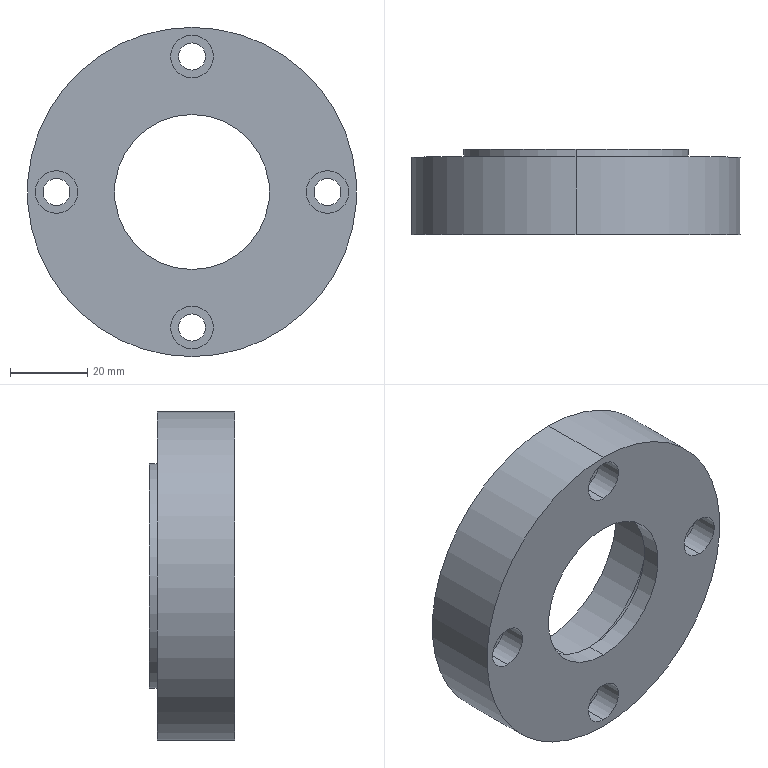Part | SolidWorks | features ICE 4, Extrusion 1, HoleWzd 1 | 1 solid | 35 faces | box 85 x 22 x 85 mm | volume 70234 mm3 | cylinder 26 | plane 9 | commonest cylinder face diameters 7 x8 11 x8 40 x2 52 x2 53.5 x2 58 x2
STEP:
#1=CARTESIAN_POINT('',(0.,-13.,40.5));
#2=VERTEX_POINT('',#1);
#3=CARTESIAN_POINT('',(0.,-13.,29.5));
#4=VERTEX_POINT('',#3);
#5=CARTESIAN_POINT('',(0.,-13.,35.));
#6=DIRECTION('',(0.,-1.,0.));
#7=DIRECTION('',(0.,0.,-1.));
#8=AXIS2_PLACEMENT_3D('',#5,#6,#7);
#9=CIRCLE('',#8,5.5);
#10=EDGE_CURVE('',#2,#4,#9,.T.);
#11=ORIENTED_EDGE('',*,*,#10,.F.);
#12=CARTESIAN_POINT('',(0.,-20.,40.5));
#13=VERTEX_POINT('',#12);
#14=CARTESIAN_POINT('',(0.,-13.,40.5));
#15=DIRECTION('',(0.,-1.,0.));
#16=VECTOR('',#15,1000.);
#17=LINE('',#14,#16);
#18=EDGE_CURVE('',#2,#13,#17,.T.);
#19=ORIENTED_EDGE('',*,*,#18,.T.);
#20=CARTESIAN_POINT('',(0.,-20.,29.5));
#21=VERTEX_POINT('',#20);
#22=CARTESIAN_POINT('',(0.,-20.,35.));
#23=DIRECTION('',(0.,-1.,0.));
#24=DIRECTION('',(0.,0.,-1.));
#25=AXIS2_PLACEMENT_3D('',#22,#23,#24);
#26=CIRCLE('',#25,5.5);
#27=EDGE_CURVE('',#13,#21,#26,.T.);
#28=ORIENTED_EDGE('',*,*,#27,.T.);
#29=CARTESIAN_POINT('',(0.,-13.,29.5));
#30=DIRECTION('',(0.,-1.,0.));
#31=VECTOR('',#30,1000.);
#32=LINE('',#29,#31);
#33=EDGE_CURVE('',#4,#21,#32,.T.);
#34=ORIENTED_EDGE('',*,*,#33,.F.);
#35=EDGE_LOOP('',(#11,#19,#28,#34));
#36=FACE_OUTER_BOUND('',#35,.T.);
#37=CARTESIAN_POINT('',(0.,-13.,35.));
#38=DIRECTION('',(0.,-1.,0.));
#39=DIRECTION('',(0.,0.,-1.));
#40=AXIS2_PLACEMENT_3D('',#37,#38,#39);
#41=CYLINDRICAL_SURFACE('',#40,5.5);
#42=ADVANCED_FACE('',(#36),#41,.F.);
#43=CARTESIAN_POINT('',(35.,-13.,5.5));
#44=VERTEX_POINT('',#43);
#45=CARTESIAN_POINT('',(35.,-13.,-5.5));
#46=VERTEX_POINT('',#45);
#47=CARTESIAN_POINT('',(35.,-13.,0.));
#48=DIRECTION('',(0.,-1.,0.));
#49=DIRECTION('',(0.,0.,-1.));
#50=AXIS2_PLACEMENT_3D('',#47,#48,#49);
#51=CIRCLE('',#50,5.5);
#52=EDGE_CURVE('',#44,#46,#51,.T.);
#53=ORIENTED_EDGE('',*,*,#52,.F.);
#54=CARTESIAN_POINT('',(35.,-20.,5.5));
#55=VERTEX_POINT('',#54);
#56=CARTESIAN_POINT('',(35.,-13.,5.5));
#57=DIRECTION('',(0.,-1.,0.));
#58=VECTOR('',#57,1000.);
#59=LINE('',#56,#58);
#60=EDGE_CURVE('',#44,#55,#59,.T.);
#61=ORIENTED_EDGE('',*,*,#60,.T.);
#62=CARTESIAN_POINT('',(35.,-20.,-5.5));
#63=VERTEX_POINT('',#62);
#64=CARTESIAN_POINT('',(35.,-20.,0.));
#65=DIRECTION('',(0.,-1.,0.));
#66=DIRECTION('',(0.,0.,-1.));
#67=AXIS2_PLACEMENT_3D('',#64,#65,#66);
#68=CIRCLE('',#67,5.5);
#69=EDGE_CURVE('',#55,#63,#68,.T.);
#70=ORIENTED_EDGE('',*,*,#69,.T.);
#71=CARTESIAN_POINT('',(35.,-13.,-5.5));
#72=DIRECTION('',(0.,-1.,0.));
#73=VECTOR('',#72,1000.);
#74=LINE('',#71,#73);
#75=EDGE_CURVE('',#46,#63,#74,.T.);
#76=ORIENTED_EDGE('',*,*,#75,.F.);
#77=EDGE_LOOP('',(#53,#61,#70,#76));
#78=FACE_OUTER_BOUND('',#77,.T.);
#79=CARTESIAN_POINT('',(35.,-13.,0.));
#80=DIRECTION('',(0.,-1.,0.));
#81=DIRECTION('',(0.,0.,-1.));
#82=AXIS2_PLACEMENT_3D('',#79,#80,#81);
#83=CYLINDRICAL_SURFACE('',#82,5.5);
#84=ADVANCED_FACE('',(#78),#83,.F.);
#85=CARTESIAN_POINT('',(-35.,-13.,5.5));
#86=VERTEX_POINT('',#85);
#87=CARTESIAN_POINT('',(-35.,-13.,-5.5));
#88=VERTEX_POINT('',#87);
#89=CARTESIAN_POINT('',(-35.,-13.,0.));
#90=DIRECTION('',(0.,-1.,0.));
#91=DIRECTION('',(0.,0.,-1.));
#92=AXIS2_PLACEMENT_3D('',#89,#90,#91);
#93=CIRCLE('',#92,5.5);
#94=EDGE_CURVE('',#86,#88,#93,.T.);
#95=ORIENTED_EDGE('',*,*,#94,.F.);
#96=CARTESIAN_POINT('',(-35.,-20.,5.5));
#97=VERTEX_POINT('',#96);
#98=CARTESIAN_POINT('',(-35.,-13.,5.5));
#99=DIRECTION('',(0.,-1.,0.));
#100=VECTOR('',#99,1000.);
#101=LINE('',#98,#100);
#102=EDGE_CURVE('',#86,#97,#101,.T.);
#103=ORIENTED_EDGE('',*,*,#102,.T.);
#104=CARTESIAN_POINT('',(-35.,-20.,-5.5));
#105=VERTEX_POINT('',#104);
#106=CARTESIAN_POINT('',(-35.,-20.,0.));
#107=DIRECTION('',(0.,-1.,0.));
#108=DIRECTION('',(0.,0.,-1.));
#109=AXIS2_PLACEMENT_3D('',#106,#107,#108);
#110=CIRCLE('',#109,5.5);
#111=EDGE_CURVE('',#97,#105,#110,.T.);
#112=ORIENTED_EDGE('',*,*,#111,.T.);
#113=CARTESIAN_POINT('',(-35.,-13.,-5.5));
#114=DIRECTION('',(0.,-1.,0.));
#115=VECTOR('',#114,1000.);
#116=LINE('',#113,#115);
#117=EDGE_CURVE('',#88,#105,#116,.T.);
#118=ORIENTED_EDGE('',*,*,#117,.F.);
#119=EDGE_LOOP('',(#95,#103,#112,#118));
#120=FACE_OUTER_BOUND('',#119,.T.);
#121=CARTESIAN_POINT('',(-35.,-13.,0.));
#122=DIRECTION('',(0.,-1.,0.));
#123=DIRECTION('',(0.,0.,-1.));
#124=AXIS2_PLACEMENT_3D('',#121,#122,#123);
#125=CYLINDRICAL_SURFACE('',#124,5.5);
#126=ADVANCED_FACE('',(#120),#125,.F.);
#127=CARTESIAN_POINT('',(0.,-13.,-29.5));
#128=VERTEX_POINT('',#127);
#129=CARTESIAN_POINT('',(0.,-13.,-40.5));
#130=VERTEX_POINT('',#129);
#131=CARTESIAN_POINT('',(0.,-13.,-35.));
#132=DIRECTION('',(0.,-1.,0.));
#133=DIRECTION('',(0.,0.,-1.));
#134=AXIS2_PLACEMENT_3D('',#131,#132,#133);
#135=CIRCLE('',#134,5.5);
#136=EDGE_CURVE('',#128,#130,#135,.T.);
#137=ORIENTED_EDGE('',*,*,#136,.F.);
#138=CARTESIAN_POINT('',(0.,-20.,-29.5));
#139=VERTEX_POINT('',#138);
#140=CARTESIAN_POINT('',(0.,-13.,-29.5));
#141=DIRECTION('',(0.,-1.,0.));
#142=VECTOR('',#141,1000.);
#143=LINE('',#140,#142);
#144=EDGE_CURVE('',#128,#139,#143,.T.);
#145=ORIENTED_EDGE('',*,*,#144,.T.);
#146=CARTESIAN_POINT('',(0.,-20.,-40.5));
#147=VERTEX_POINT('',#146);
#148=CARTESIAN_POINT('',(0.,-20.,-35.));
#149=DIRECTION('',(0.,-1.,0.));
#150=DIRECTION('',(0.,0.,-1.));
#151=AXIS2_PLACEMENT_3D('',#148,#149,#150);
#152=CIRCLE('',#151,5.5);
#153=EDGE_CURVE('',#139,#147,#152,.T.);
#154=ORIENTED_EDGE('',*,*,#153,.T.);
#155=CARTESIAN_POINT('',(0.,-13.,-40.5));
#156=DIRECTION('',(0.,-1.,0.));
#157=VECTOR('',#156,1000.);
#158=LINE('',#155,#157);
#159=EDGE_CURVE('',#130,#147,#158,.T.);
#160=ORIENTED_EDGE('',*,*,#159,.F.);
#161=EDGE_LOOP('',(#137,#145,#154,#160));
#162=FACE_OUTER_BOUND('',#161,.T.);
#163=CARTESIAN_POINT('',(0.,-13.,-35.));
#164=DIRECTION('',(0.,-1.,0.));
#165=DIRECTION('',(0.,0.,-1.));
#166=AXIS2_PLACEMENT_3D('',#163,#164,#165);
#167=CYLINDRICAL_SURFACE('',#166,5.5);
#168=ADVANCED_FACE('',(#162),#167,.F.);
#169=CARTESIAN_POINT('',(0.,2.,-26.75));
#170=VERTEX_POINT('',#169);
#171=CARTESIAN_POINT('',(0.,2.,26.75));
#172=VERTEX_POINT('',#171);
#173=CARTESIAN_POINT('',(0.,2.,0.));
#174=DIRECTION('',(0.,1.,0.));
#175=DIRECTION('',(0.,0.,1.));
#176=AXIS2_PLACEMENT_3D('',#173,#174,#175);
#177=CIRCLE('',#176,26.75);
#178=EDGE_CURVE('',#170,#172,#177,.T.);
#179=ORIENTED_EDGE('',*,*,#178,.T.);
#180=CARTESIAN_POINT('',(0.,-10.,26.75));
#181=VERTEX_POINT('',#180);
#182=CARTESIAN_POINT('',(0.,2.,26.75));
#183=DIRECTION('',(0.,-1.,0.));
#184=VECTOR('',#183,1000.);
#185=LINE('',#182,#184);
#186=EDGE_CURVE('',#172,#181,#185,.T.);
#187=ORIENTED_EDGE('',*,*,#186,.T.);
#188=CARTESIAN_POINT('',(0.,-10.,-26.75));
#189=VERTEX_POINT('',#188);
#190=CARTESIAN_POINT('',(0.,-10.,0.));
#191=DIRECTION('',(0.,1.,0.));
#192=DIRECTION('',(0.,0.,1.));
#193=AXIS2_PLACEMENT_3D('',#190,#191,#192);
#194=CIRCLE('',#193,26.75);
#195=EDGE_CURVE('',#189,#181,#194,.T.);
#196=ORIENTED_EDGE('',*,*,#195,.F.);
#197=CARTESIAN_POINT('',(0.,2.,-26.75));
#198=DIRECTION('',(0.,-1.,0.));
#199=VECTOR('',#198,1000.);
#200=LINE('',#197,#199);
#201=EDGE_CURVE('',#170,#189,#200,.T.);
#202=ORIENTED_EDGE('',*,*,#201,.F.);
#203=EDGE_LOOP('',(#179,#187,#196,#202));
#204=FACE_OUTER_BOUND('',#203,.T.);
#205=CARTESIAN_POINT('',(0.,2.,0.));
#206=DIRECTION('',(0.,-1.,0.));
#207=DIRECTION('',(0.,0.,-1.));
#208=AXIS2_PLACEMENT_3D('',#205,#206,#207);
#209=CYLINDRICAL_SURFACE('',#208,26.75);
#210=ADVANCED_FACE('',(#204),#209,.F.);
#211=CARTESIAN_POINT('',(0.,2.,29.));
#212=VERTEX_POINT('',#211);
#213=CARTESIAN_POINT('',(0.,2.,-29.));
#214=VERTEX_POINT('',#213);
#215=CARTESIAN_POINT('',(0.,2.,0.));
#216=DIRECTION('',(0.,1.,0.));
#217=DIRECTION('',(0.,0.,1.));
#218=AXIS2_PLACEMENT_3D('',#215,#216,#217);
#219=CIRCLE('',#218,29.);
#220=EDGE_CURVE('',#212,#214,#219,.T.);
#221=ORIENTED_EDGE('',*,*,#220,.F.);
#222=CARTESIAN_POINT('',(0.,0.,29.));
#223=VERTEX_POINT('',#222);
#224=CARTESIAN_POINT('',(0.,2.,29.));
#225=DIRECTION('',(0.,-1.,0.));
#226=VECTOR('',#225,1000.);
#227=LINE('',#224,#226);
#228=EDGE_CURVE('',#212,#223,#227,.T.);
#229=ORIENTED_EDGE('',*,*,#228,.T.);
#230=CARTESIAN_POINT('',(0.,0.,-29.));
#231=VERTEX_POINT('',#230);
#232=CARTESIAN_POINT('',(0.,0.,0.));
#233=DIRECTION('',(0.,1.,0.));
#234=DIRECTION('',(0.,0.,-1.));
#235=AXIS2_PLACEMENT_3D('',#232,#233,#234);
#236=CIRCLE('',#235,29.);
#237=EDGE_CURVE('',#223,#231,#236,.T.);
#238=ORIENTED_EDGE('',*,*,#237,.T.);
#239=CARTESIAN_POINT('',(0.,2.,-29.));
#240=DIRECTION('',(0.,-1.,0.));
#241=VECTOR('',#240,1000.);
#242=LINE('',#239,#241);
#243=EDGE_CURVE('',#214,#231,#242,.T.);
#244=ORIENTED_EDGE('',*,*,#243,.F.);
#245=EDGE_LOOP('',(#221,#229,#238,#244));
#246=FACE_OUTER_BOUND('',#245,.T.);
#247=CARTESIAN_POINT('',(0.,2.,0.));
#248=DIRECTION('',(0.,-1.,0.));
#249=DIRECTION('',(0.,0.,-1.));
#250=AXIS2_PLACEMENT_3D('',#247,#248,#249);
#251=CYLINDRICAL_SURFACE('',#250,29.);
#252=ADVANCED_FACE('',(#246),#251,.T.);
#253=CARTESIAN_POINT('',(0.,-20.,-42.5));
#254=VERTEX_POINT('',#253);
#255=CARTESIAN_POINT('',(0.,-20.,42.5));
#256=VERTEX_POINT('',#255);
#257=CARTESIAN_POINT('',(0.,-20.,0.));
#258=DIRECTION('',(0.,-1.,0.));
#259=DIRECTION('',(0.,0.,-1.));
#260=AXIS2_PLACEMENT_3D('',#257,#258,#259);
#261=CIRCLE('',#260,42.5);
#262=EDGE_CURVE('',#254,#256,#261,.T.);
#263=ORIENTED_EDGE('',*,*,#262,.F.);
#264=CARTESIAN_POINT('',(0.,0.,-42.5));
#265=VERTEX_POINT('',#264);
#266=CARTESIAN_POINT('',(0.,-20.,-42.5));
#267=DIRECTION('',(0.,1.,0.));
#268=VECTOR('',#267,1000.);
#269=LINE('',#266,#268);
#270=EDGE_CURVE('',#254,#265,#269,.T.);
#271=ORIENTED_EDGE('',*,*,#270,.T.);
#272=CARTESIAN_POINT('',(0.,0.,42.5));
#273=VERTEX_POINT('',#272);
#274=CARTESIAN_POINT('',(0.,0.,0.));
#275=DIRECTION('',(0.,-1.,0.));
#276=DIRECTION('',(0.,0.,-1.));
#277=AXIS2_PLACEMENT_3D('',#274,#275,#276);
#278=CIRCLE('',#277,42.5);
#279=EDGE_CURVE('',#265,#273,#278,.T.);
#280=ORIENTED_EDGE('',*,*,#279,.T.);
#281=CARTESIAN_POINT('',(0.,-20.,42.5));
#282=DIRECTION('',(0.,1.,0.));
#283=VECTOR('',#282,1000.);
#284=LINE('',#281,#283);
#285=EDGE_CURVE('',#256,#273,#284,.T.);
#286=ORIENTED_EDGE('',*,*,#285,.F.);
#287=EDGE_LOOP('',(#263,#271,#280,#286));
#288=FACE_OUTER_BOUND('',#287,.T.);
#289=CARTESIAN_POINT('',(0.,-20.,0.));
#290=DIRECTION('',(0.,1.,0.));
#291=DIRECTION('',(0.,0.,1.));
#292=AXIS2_PLACEMENT_3D('',#289,#290,#291);
#293=CYLINDRICAL_SURFACE('',#292,42.5);
#294=ADVANCED_FACE('',(#288),#293,.T.);
#295=CARTESIAN_POINT('',(0.,-20.,20.));
#296=VERTEX_POINT('',#295);
#297=CARTESIAN_POINT('',(0.,-20.,-20.));
#298=VERTEX_POINT('',#297);
#299=CARTESIAN_POINT('',(0.,-20.,0.));
#300=DIRECTION('',(0.,-1.,0.));
#301=DIRECTION('',(0.,0.,-1.));
#302=AXIS2_PLACEMENT_3D('',#299,#300,#301);
#303=CIRCLE('',#302,20.);
#304=EDGE_CURVE('',#296,#298,#303,.T.);
#305=ORIENTED_EDGE('',*,*,#304,.T.);
#306=CARTESIAN_POINT('',(0.,-15.,-20.));
#307=VERTEX_POINT('',#306);
#308=CARTESIAN_POINT('',(0.,-20.,-20.));
#309=DIRECTION('',(0.,1.,0.));
#310=VECTOR('',#309,1000.);
#311=LINE('',#308,#310);
#312=EDGE_CURVE('',#298,#307,#311,.T.);
#313=ORIENTED_EDGE('',*,*,#312,.T.);
#314=CARTESIAN_POINT('',(0.,-15.,20.));
#315=VERTEX_POINT('',#314);
#316=CARTESIAN_POINT('',(0.,-15.,0.));
#317=DIRECTION('',(0.,1.,0.));
#318=DIRECTION('',(0.,0.,1.));
#319=AXIS2_PLACEMENT_3D('',#316,#317,#318);
#320=CIRCLE('',#319,20.);
#321=EDGE_CURVE('',#307,#315,#320,.T.);
#322=ORIENTED_EDGE('',*,*,#321,.T.);
#323=CARTESIAN_POINT('',(0.,-20.,20.));
#324=DIRECTION('',(0.,1.,0.));
#325=VECTOR('',#324,1000.);
#326=LINE('',#323,#325);
#327=EDGE_CURVE('',#296,#315,#326,.T.);
#328=ORIENTED_EDGE('',*,*,#327,.F.);
#329=EDGE_LOOP('',(#305,#313,#322,#328));
#330=FACE_OUTER_BOUND('',#329,.T.);
#331=CARTESIAN_POINT('',(0.,-20.,0.));
#332=DIRECTION('',(0.,1.,0.));
#333=DIRECTION('',(0.,0.,1.));
#334=AXIS2_PLACEMENT_3D('',#331,#332,#333);
#335=CYLINDRICAL_SURFACE('',#334,20.);
#336=ADVANCED_FACE('',(#330),#335,.F.);
#337=CARTESIAN_POINT('',(0.,-15.,-26.));
#338=VERTEX_POINT('',#337);
#339=CARTESIAN_POINT('',(0.,-15.,26.));
#340=VERTEX_POINT('',#339);
#341=CARTESIAN_POINT('',(0.,-15.,0.));
#342=DIRECTION('',(0.,1.,0.));
#343=DIRECTION('',(0.,0.,1.));
#344=AXIS2_PLACEMENT_3D('',#341,#342,#343);
#345=CIRCLE('',#344,26.);
#346=EDGE_CURVE('',#338,#340,#345,.T.);
#347=ORIENTED_EDGE('',*,*,#346,.F.);
#348=CARTESIAN_POINT('',(0.,-10.,-26.));
#349=VERTEX_POINT('',#348);
#350=CARTESIAN_POINT('',(0.,-15.,-26.));
#351=DIRECTION('',(0.,1.,0.));
#352=VECTOR('',#351,1000.);
#353=LINE('',#350,#352);
#354=EDGE_CURVE('',#338,#349,#353,.T.);
#355=ORIENTED_EDGE('',*,*,#354,.T.);
#356=CARTESIAN_POINT('',(0.,-10.,26.));
#357=VERTEX_POINT('',#356);
#358=CARTESIAN_POINT('',(0.,-10.,0.));
#359=DIRECTION('',(0.,-1.,0.));
#360=DIRECTION('',(0.,0.,1.));
#361=AXIS2_PLACEMENT_3D('',#358,#359,#360);
#362=CIRCLE('',#361,26.);
#363=EDGE_CURVE('',#357,#349,#362,.T.);
#364=ORIENTED_EDGE('',*,*,#363,.F.);
#365=CARTESIAN_POINT('',(0.,-15.,26.));
#366=DIRECTION('',(0.,1.,0.));
#367=VECTOR('',#366,1000.);
#368=LINE('',#365,#367);
#369=EDGE_CURVE('',#340,#357,#368,.T.);
#370=ORIENTED_EDGE('',*,*,#369,.F.);
#371=EDGE_LOOP('',(#347,#355,#364,#370));
#372=FACE_OUTER_BOUND('',#371,.T.);
#373=CARTESIAN_POINT('',(0.,-15.,0.));
#374=DIRECTION('',(0.,1.,0.));
#375=DIRECTION('',(0.,0.,1.));
#376=AXIS2_PLACEMENT_3D('',#373,#374,#375);
#377=CYLINDRICAL_SURFACE('',#376,26.);
#378=ADVANCED_FACE('',(#372),#377,.F.);
#379=CARTESIAN_POINT('',(0.,-13.,-38.5));
#380=VERTEX_POINT('',#379);
#381=CARTESIAN_POINT('',(0.,-13.,-31.5));
#382=VERTEX_POINT('',#381);
#383=CARTESIAN_POINT('',(0.,-13.,-35.));
#384=DIRECTION('',(0.,1.,0.));
#385=DIRECTION('',(0.,0.,-1.));
#386=AXIS2_PLACEMENT_3D('',#383,#384,#385);
#387=CIRCLE('',#386,3.5);
#388=EDGE_CURVE('',#380,#382,#387,.T.);
#389=ORIENTED_EDGE('',*,*,#388,.F.);
#390=CARTESIAN_POINT('',(0.,0.,-38.5));
#391=VERTEX_POINT('',#390);
#392=CARTESIAN_POINT('',(0.,0.,-38.5));
#393=DIRECTION('',(0.,1.,0.));
#394=VECTOR('',#393,1000.);
#395=LINE('',#392,#394);
#396=EDGE_CURVE('',#380,#391,#395,.T.);
#397=ORIENTED_EDGE('',*,*,#396,.T.);
#398=CARTESIAN_POINT('',(0.,0.,-31.5));
#399=VERTEX_POINT('',#398);
#400=CARTESIAN_POINT('',(0.,0.,-35.));
#401=DIRECTION('',(0.,1.,0.));
#402=DIRECTION('',(0.,0.,1.));
#403=AXIS2_PLACEMENT_3D('',#400,#401,#402);
#404=CIRCLE('',#403,3.5);
#405=EDGE_CURVE('',#391,#399,#404,.T.);
#406=ORIENTED_EDGE('',*,*,#405,.T.);
#407=CARTESIAN_POINT('',(0.,0.,-31.5));
#408=DIRECTION('',(0.,1.,0.));
#409=VECTOR('',#408,1000.);
#410=LINE('',#407,#409);
#411=EDGE_CURVE('',#382,#399,#410,.T.);
#412=ORIENTED_EDGE('',*,*,#411,.F.);
#413=EDGE_LOOP('',(#389,#397,#406,#412));
#414=FACE_OUTER_BOUND('',#413,.T.);
#415=CARTESIAN_POINT('',(0.,0.,-35.));
#416=DIRECTION('',(0.,1.,0.));
#417=DIRECTION('',(0.,0.,1.));
#418=AXIS2_PLACEMENT_3D('',#415,#416,#417);
#419=CYLINDRICAL_SURFACE('',#418,3.5);
#420=ADVANCED_FACE('',(#414),#419,.F.);
#421=CARTESIAN_POINT('',(-35.,-13.,-3.5));
#422=VERTEX_POINT('',#421);
#423=CARTESIAN_POINT('',(-35.,-13.,3.5));
#424=VERTEX_POINT('',#423);
#425=CARTESIAN_POINT('',(-35.,-13.,0.));
#426=DIRECTION('',(0.,1.,0.));
#427=DIRECTION('',(0.,0.,-1.));
#428=AXIS2_PLACEMENT_3D('',#425,#426,#427);
#429=CIRCLE('',#428,3.5);
#430=EDGE_CURVE('',#422,#424,#429,.T.);
#431=ORIENTED_EDGE('',*,*,#430,.F.);
#432=CARTESIAN_POINT('',(-35.,0.,-3.5));
#433=VERTEX_POINT('',#432);
#434=CARTESIAN_POINT('',(-35.,0.,-3.5));
#435=DIRECTION('',(0.,1.,0.));
#436=VECTOR('',#435,1000.);
#437=LINE('',#434,#436);
#438=EDGE_CURVE('',#422,#433,#437,.T.);
#439=ORIENTED_EDGE('',*,*,#438,.T.);
#440=CARTESIAN_POINT('',(-35.,0.,3.5));
#441=VERTEX_POINT('',#440);
#442=CARTESIAN_POINT('',(-35.,0.,0.));
#443=DIRECTION('',(0.,1.,0.));
#444=DIRECTION('',(0.,0.,1.));
#445=AXIS2_PLACEMENT_3D('',#442,#443,#444);
#446=CIRCLE('',#445,3.5);
#447=EDGE_CURVE('',#433,#441,#446,.T.);
#448=ORIENTED_EDGE('',*,*,#447,.T.);
#449=CARTESIAN_POINT('',(-35.,0.,3.5));
#450=DIRECTION('',(0.,1.,0.));
#451=VECTOR('',#450,1000.);
#452=LINE('',#449,#451);
#453=EDGE_CURVE('',#424,#441,#452,.T.);
#454=ORIENTED_EDGE('',*,*,#453,.F.);
#455=EDGE_LOOP('',(#431,#439,#448,#454));
#456=FACE_OUTER_BOUND('',#455,.T.);
#457=CARTESIAN_POINT('',(-35.,0.,0.));
#458=DIRECTION('',(0.,1.,0.));
#459=DIRECTION('',(0.,0.,1.));
#460=AXIS2_PLACEMENT_3D('',#457,#458,#459);
#461=CYLINDRICAL_SURFACE('',#460,3.5);
#462=ADVANCED_FACE('',(#456),#461,.F.);
#463=CARTESIAN_POINT('',(35.,-13.,-3.5));
#464=VERTEX_POINT('',#463);
#465=CARTESIAN_POINT('',(35.,-13.,3.5));
#466=VERTEX_POINT('',#465);
#467=CARTESIAN_POINT('',(35.,-13.,0.));
#468=DIRECTION('',(0.,1.,0.));
#469=DIRECTION('',(0.,0.,-1.));
#470=AXIS2_PLACEMENT_3D('',#467,#468,#469);
#471=CIRCLE('',#470,3.5);
#472=EDGE_CURVE('',#464,#466,#471,.T.);
#473=ORIENTED_EDGE('',*,*,#472,.F.);
#474=CARTESIAN_POINT('',(35.,0.,-3.5));
#475=VERTEX_POINT('',#474);
#476=CARTESIAN_POINT('',(35.,0.,-3.5));
#477=DIRECTION('',(0.,1.,0.));
#478=VECTOR('',#477,1000.);
#479=LINE('',#476,#478);
#480=EDGE_CURVE('',#464,#475,#479,.T.);
#481=ORIENTED_EDGE('',*,*,#480,.T.);
#482=CARTESIAN_POINT('',(35.,0.,3.5));
#483=VERTEX_POINT('',#482);
#484=CARTESIAN_POINT('',(35.,0.,0.));
#485=DIRECTION('',(0.,1.,0.));
#486=DIRECTION('',(0.,0.,1.));
#487=AXIS2_PLACEMENT_3D('',#484,#485,#486);
#488=CIRCLE('',#487,3.5);
#489=EDGE_CURVE('',#475,#483,#488,.T.);
#490=ORIENTED_EDGE('',*,*,#489,.T.);
#491=CARTESIAN_POINT('',(35.,0.,3.5));
#492=DIRECTION('',(0.,1.,0.));
#493=VECTOR('',#492,1000.);
#494=LINE('',#491,#493);
#495=EDGE_CURVE('',#466,#483,#494,.T.);
#496=ORIENTED_EDGE('',*,*,#495,.F.);
#497=EDGE_LOOP('',(#473,#481,#490,#496));
#498=FACE_OUTER_BOUND('',#497,.T.);
#499=CARTESIAN_POINT('',(35.,0.,0.));
#500=DIRECTION('',(0.,1.,0.));
#501=DIRECTION('',(0.,0.,1.));
#502=AXIS2_PLACEMENT_3D('',#499,#500,#501);
#503=CYLINDRICAL_SURFACE('',#502,3.5);
#504=ADVANCED_FACE('',(#498),#503,.F.);
#505=CARTESIAN_POINT('',(0.,-13.,31.5));
#506=VERTEX_POINT('',#505);
#507=CARTESIAN_POINT('',(0.,-13.,38.5));
#508=VERTEX_POINT('',#507);
#509=CARTESIAN_POINT('',(0.,-13.,35.));
#510=DIRECTION('',(0.,1.,0.));
#511=DIRECTION('',(0.,0.,-1.));
#512=AXIS2_PLACEMENT_3D('',#509,#510,#511);
#513=CIRCLE('',#512,3.5);
#514=EDGE_CURVE('',#506,#508,#513,.T.);
#515=ORIENTED_EDGE('',*,*,#514,.F.);
#516=CARTESIAN_POINT('',(0.,0.,31.5));
#517=VERTEX_POINT('',#516);
#518=CARTESIAN_POINT('',(0.,0.,31.5));
#519=DIRECTION('',(0.,1.,0.));
#520=VECTOR('',#519,1000.);
#521=LINE('',#518,#520);
#522=EDGE_CURVE('',#506,#517,#521,.T.);
#523=ORIENTED_EDGE('',*,*,#522,.T.);
#524=CARTESIAN_POINT('',(0.,0.,38.5));
#525=VERTEX_POINT('',#524);
#526=CARTESIAN_POINT('',(0.,0.,35.));
#527=DIRECTION('',(0.,1.,0.));
#528=DIRECTION('',(0.,0.,1.));
#529=AXIS2_PLACEMENT_3D('',#526,#527,#528);
#530=CIRCLE('',#529,3.5);
#531=EDGE_CURVE('',#517,#525,#530,.T.);
#532=ORIENTED_EDGE('',*,*,#531,.T.);
#533=CARTESIAN_POINT('',(0.,0.,38.5));
#534=DIRECTION('',(0.,1.,0.));
#535=VECTOR('',#534,1000.);
#536=LINE('',#533,#535);
#537=EDGE_CURVE('',#508,#525,#536,.T.);
#538=ORIENTED_EDGE('',*,*,#537,.F.);
#539=EDGE_LOOP('',(#515,#523,#532,#538));
#540=FACE_OUTER_BOUND('',#539,.T.);
#541=CARTESIAN_POINT('',(0.,0.,35.));
#542=DIRECTION('',(0.,1.,0.));
#543=DIRECTION('',(0.,0.,1.));
#544=AXIS2_PLACEMENT_3D('',#541,#542,#543);
#545=CYLINDRICAL_SURFACE('',#544,3.5);
#546=ADVANCED_FACE('',(#540),#545,.F.);
#547=ORIENTED_EDGE('',*,*,#522,.F.);
#548=CARTESIAN_POINT('',(0.,-13.,35.));
#549=DIRECTION('',(0.,1.,0.));
#550=DIRECTION('',(0.,0.,-1.));
#551=AXIS2_PLACEMENT_3D('',#548,#549,#550);
#552=CIRCLE('',#551,3.5);
#553=EDGE_CURVE('',#508,#506,#552,.T.);
#554=ORIENTED_EDGE('',*,*,#553,.F.);
#555=ORIENTED_EDGE('',*,*,#537,.T.);
#556=CARTESIAN_POINT('',(0.,0.,35.));
#557=DIRECTION('',(0.,1.,0.));
#558=DIRECTION('',(0.,0.,1.));
#559=AXIS2_PLACEMENT_3D('',#556,#557,#558);
#560=CIRCLE('',#559,3.5);
#561=EDGE_CURVE('',#525,#517,#560,.T.);
#562=ORIENTED_EDGE('',*,*,#561,.T.);
#563=EDGE_LOOP('',(#547,#554,#555,#562));
#564=FACE_OUTER_BOUND('',#563,.T.);
#565=CARTESIAN_POINT('',(0.,0.,35.));
#566=DIRECTION('',(0.,1.,0.));
#567=DIRECTION('',(0.,0.,1.));
#568=AXIS2_PLACEMENT_3D('',#565,#566,#567);
#569=CYLINDRICAL_SURFACE('',#568,3.5);
#570=ADVANCED_FACE('',(#564),#569,.F.);
#571=ORIENTED_EDGE('',*,*,#480,.F.);
#572=CARTESIAN_POINT('',(35.,-13.,0.));
#573=DIRECTION('',(0.,1.,0.));
#574=DIRECTION('',(0.,0.,-1.));
#575=AXIS2_PLACEMENT_3D('',#572,#573,#574);
#576=CIRCLE('',#575,3.5);
#577=EDGE_CURVE('',#466,#464,#576,.T.);
#578=ORIENTED_EDGE('',*,*,#577,.F.);
#579=ORIENTED_EDGE('',*,*,#495,.T.);
#580=CARTESIAN_POINT('',(35.,0.,0.));
#581=DIRECTION('',(0.,1.,0.));
#582=DIRECTION('',(0.,0.,1.));
#583=AXIS2_PLACEMENT_3D('',#580,#581,#582);
#584=CIRCLE('',#583,3.5);
#585=EDGE_CURVE('',#483,#475,#584,.T.);
#586=ORIENTED_EDGE('',*,*,#585,.T.);
#587=EDGE_LOOP('',(#571,#578,#579,#586));
#588=FACE_OUTER_BOUND('',#587,.T.);
#589=CARTESIAN_POINT('',(35.,0.,0.));
#590=DIRECTION('',(0.,1.,0.));
#591=DIRECTION('',(0.,0.,1.));
#592=AXIS2_PLACEMENT_3D('',#589,#590,#591);
#593=CYLINDRICAL_SURFACE('',#592,3.5);
#594=ADVANCED_FACE('',(#588),#593,.F.);
#595=ORIENTED_EDGE('',*,*,#438,.F.);
#596=CARTESIAN_POINT('',(-35.,-13.,0.));
#597=DIRECTION('',(0.,1.,0.));
#598=DIRECTION('',(0.,0.,-1.));
#599=AXIS2_PLACEMENT_3D('',#596,#597,#598);
#600=CIRCLE('',#599,3.5);
#601=EDGE_CURVE('',#424,#422,#600,.T.);
#602=ORIENTED_EDGE('',*,*,#601,.F.);
#603=ORIENTED_EDGE('',*,*,#453,.T.);
#604=CARTESIAN_POINT('',(-35.,0.,0.));
#605=DIRECTION('',(0.,1.,0.));
#606=DIRECTION('',(0.,0.,1.));
#607=AXIS2_PLACEMENT_3D('',#604,#605,#606);
#608=CIRCLE('',#607,3.5);
#609=EDGE_CURVE('',#441,#433,#608,.T.);
#610=ORIENTED_EDGE('',*,*,#609,.T.);
#611=EDGE_LOOP('',(#595,#602,#603,#610));
#612=FACE_OUTER_BOUND('',#611,.T.);
#613=CARTESIAN_POINT('',(-35.,0.,0.));
#614=DIRECTION('',(0.,1.,0.));
#615=DIRECTION('',(0.,0.,1.));
#616=AXIS2_PLACEMENT_3D('',#613,#614,#615);
#617=CYLINDRICAL_SURFACE('',#616,3.5);
#618=ADVANCED_FACE('',(#612),#617,.F.);
#619=ORIENTED_EDGE('',*,*,#396,.F.);
#620=CARTESIAN_POINT('',(0.,-13.,-35.));
#621=DIRECTION('',(0.,1.,0.));
#622=DIRECTION('',(0.,0.,-1.));
#623=AXIS2_PLACEMENT_3D('',#620,#621,#622);
#624=CIRCLE('',#623,3.5);
#625=EDGE_CURVE('',#382,#380,#624,.T.);
#626=ORIENTED_EDGE('',*,*,#625,.F.);
#627=ORIENTED_EDGE('',*,*,#411,.T.);
#628=CARTESIAN_POINT('',(0.,0.,-35.));
#629=DIRECTION('',(0.,1.,0.));
#630=DIRECTION('',(0.,0.,1.));
#631=AXIS2_PLACEMENT_3D('',#628,#629,#630);
#632=CIRCLE('',#631,3.5);
#633=EDGE_CURVE('',#399,#391,#632,.T.);
#634=ORIENTED_EDGE('',*,*,#633,.T.);
#635=EDGE_LOOP('',(#619,#626,#627,#634));
#636=FACE_OUTER_BOUND('',#635,.T.);
#637=CARTESIAN_POINT('',(0.,0.,-35.));
#638=DIRECTION('',(0.,1.,0.));
#639=DIRECTION('',(0.,0.,1.));
#640=AXIS2_PLACEMENT_3D('',#637,#638,#639);
#641=CYLINDRICAL_SURFACE('',#640,3.5);
#642=ADVANCED_FACE('',(#636),#641,.F.);
#643=ORIENTED_EDGE('',*,*,#354,.F.);
#644=CARTESIAN_POINT('',(0.,-15.,0.));
#645=DIRECTION('',(0.,1.,0.));
#646=DIRECTION('',(0.,0.,1.));
#647=AXIS2_PLACEMENT_3D('',#644,#645,#646);
#648=CIRCLE('',#647,26.);
#649=EDGE_CURVE('',#340,#338,#648,.T.);
#650=ORIENTED_EDGE('',*,*,#649,.F.);
#651=ORIENTED_EDGE('',*,*,#369,.T.);
#652=CARTESIAN_POINT('',(0.,-10.,0.));
#653=DIRECTION('',(0.,-1.,0.));
#654=DIRECTION('',(0.,0.,1.));
#655=AXIS2_PLACEMENT_3D('',#652,#653,#654);
#656=CIRCLE('',#655,26.);
#657=EDGE_CURVE('',#349,#357,#656,.T.);
#658=ORIENTED_EDGE('',*,*,#657,.F.);
#659=EDGE_LOOP('',(#643,#650,#651,#658));
#660=FACE_OUTER_BOUND('',#659,.T.);
#661=CARTESIAN_POINT('',(0.,-15.,0.));
#662=DIRECTION('',(0.,1.,0.));
#663=DIRECTION('',(0.,0.,1.));
#664=AXIS2_PLACEMENT_3D('',#661,#662,#663);
#665=CYLINDRICAL_SURFACE('',#664,26.);
#666=ADVANCED_FACE('',(#660),#665,.F.);
#667=ORIENTED_EDGE('',*,*,#312,.F.);
#668=CARTESIAN_POINT('',(0.,-20.,0.));
#669=DIRECTION('',(0.,-1.,0.));
#670=DIRECTION('',(0.,0.,-1.));
#671=AXIS2_PLACEMENT_3D('',#668,#669,#670);
#672=CIRCLE('',#671,20.);
#673=EDGE_CURVE('',#298,#296,#672,.T.);
#674=ORIENTED_EDGE('',*,*,#673,.T.);
#675=ORIENTED_EDGE('',*,*,#327,.T.);
#676=CARTESIAN_POINT('',(0.,-15.,0.));
#677=DIRECTION('',(0.,1.,0.));
#678=DIRECTION('',(0.,0.,1.));
#679=AXIS2_PLACEMENT_3D('',#676,#677,#678);
#680=CIRCLE('',#679,20.);
#681=EDGE_CURVE('',#315,#307,#680,.T.);
#682=ORIENTED_EDGE('',*,*,#681,.T.);
#683=EDGE_LOOP('',(#667,#674,#675,#682));
#684=FACE_OUTER_BOUND('',#683,.T.);
#685=CARTESIAN_POINT('',(0.,-20.,0.));
#686=DIRECTION('',(0.,1.,0.));
#687=DIRECTION('',(0.,0.,1.));
#688=AXIS2_PLACEMENT_3D('',#685,#686,#687);
#689=CYLINDRICAL_SURFACE('',#688,20.);
#690=ADVANCED_FACE('',(#684),#689,.F.);
#691=CARTESIAN_POINT('',(0.,-20.,35.));
#692=DIRECTION('',(0.,-1.,0.));
#693=DIRECTION('',(0.,0.,-1.));
#694=AXIS2_PLACEMENT_3D('',#691,#692,#693);
#695=CIRCLE('',#694,5.5);
#696=EDGE_CURVE('',#21,#13,#695,.T.);
#697=ORIENTED_EDGE('',*,*,#696,.F.);
#698=ORIENTED_EDGE('',*,*,#27,.F.);
#699=EDGE_LOOP('',(#697,#698));
#700=FACE_BOUND('',#699,.T.);
#701=CARTESIAN_POINT('',(-35.,-20.,0.));
#702=DIRECTION('',(0.,-1.,0.));
#703=DIRECTION('',(0.,0.,-1.));
#704=AXIS2_PLACEMENT_3D('',#701,#702,#703);
#705=CIRCLE('',#704,5.5);
#706=EDGE_CURVE('',#105,#97,#705,.T.);
#707=ORIENTED_EDGE('',*,*,#706,.F.);
#708=ORIENTED_EDGE('',*,*,#111,.F.);
#709=EDGE_LOOP('',(#707,#708));
#710=FACE_BOUND('',#709,.T.);
#711=CARTESIAN_POINT('',(0.,-20.,-35.));
#712=DIRECTION('',(0.,-1.,0.));
#713=DIRECTION('',(0.,0.,-1.));
#714=AXIS2_PLACEMENT_3D('',#711,#712,#713);
#715=CIRCLE('',#714,5.5);
#716=EDGE_CURVE('',#147,#139,#715,.T.);
#717=ORIENTED_EDGE('',*,*,#716,.F.);
#718=ORIENTED_EDGE('',*,*,#153,.F.);
#719=EDGE_LOOP('',(#717,#718));
#720=FACE_BOUND('',#719,.T.);
#721=CARTESIAN_POINT('',(35.,-20.,0.));
#722=DIRECTION('',(0.,-1.,0.));
#723=DIRECTION('',(0.,0.,-1.));
#724=AXIS2_PLACEMENT_3D('',#721,#722,#723);
#725=CIRCLE('',#724,5.5);
#726=EDGE_CURVE('',#63,#55,#725,.T.);
#727=ORIENTED_EDGE('',*,*,#726,.F.);
#728=ORIENTED_EDGE('',*,*,#69,.F.);
#729=EDGE_LOOP('',(#727,#728));
#730=FACE_BOUND('',#729,.T.);
#731=CARTESIAN_POINT('',(0.,-20.,0.));
#732=DIRECTION('',(0.,-1.,0.));
#733=DIRECTION('',(0.,0.,-1.));
#734=AXIS2_PLACEMENT_3D('',#731,#732,#733);
#735=CIRCLE('',#734,42.5);
#736=EDGE_CURVE('',#256,#254,#735,.T.);
#737=ORIENTED_EDGE('',*,*,#736,.T.);
#738=ORIENTED_EDGE('',*,*,#262,.T.);
#739=EDGE_LOOP('',(#737,#738));
#740=FACE_OUTER_BOUND('',#739,.T.);
#741=ORIENTED_EDGE('',*,*,#304,.F.);
#742=ORIENTED_EDGE('',*,*,#673,.F.);
#743=EDGE_LOOP('',(#741,#742));
#744=FACE_BOUND('',#743,.T.);
#745=CARTESIAN_POINT('',(0.,-20.,0.));
#746=DIRECTION('',(0.,-1.,0.));
#747=DIRECTION('',(0.,0.,-1.));
#748=AXIS2_PLACEMENT_3D('',#745,#746,#747);
#749=PLANE('',#748);
#750=ADVANCED_FACE('',(#700,#710,#720,#730,#740,#744),#749,.T.);
#751=CARTESIAN_POINT('',(0.,0.,0.));
#752=DIRECTION('',(0.,1.,0.));
#753=DIRECTION('',(0.,0.,-1.));
#754=AXIS2_PLACEMENT_3D('',#751,#752,#753);
#755=CIRCLE('',#754,29.);
#756=EDGE_CURVE('',#231,#223,#755,.T.);
#757=ORIENTED_EDGE('',*,*,#756,.F.);
#758=ORIENTED_EDGE('',*,*,#237,.F.);
#759=EDGE_LOOP('',(#757,#758));
#760=FACE_BOUND('',#759,.T.);
#761=ORIENTED_EDGE('',*,*,#633,.F.);
#762=ORIENTED_EDGE('',*,*,#405,.F.);
#763=EDGE_LOOP('',(#761,#762));
#764=FACE_BOUND('',#763,.T.);
#765=ORIENTED_EDGE('',*,*,#609,.F.);
#766=ORIENTED_EDGE('',*,*,#447,.F.);
#767=EDGE_LOOP('',(#765,#766));
#768=FACE_BOUND('',#767,.T.);
#769=ORIENTED_EDGE('',*,*,#585,.F.);
#770=ORIENTED_EDGE('',*,*,#489,.F.);
#771=EDGE_LOOP('',(#769,#770));
#772=FACE_BOUND('',#771,.T.);
#773=ORIENTED_EDGE('',*,*,#561,.F.);
#774=ORIENTED_EDGE('',*,*,#531,.F.);
#775=EDGE_LOOP('',(#773,#774));
#776=FACE_BOUND('',#775,.T.);
#777=CARTESIAN_POINT('',(0.,0.,0.));
#778=DIRECTION('',(0.,-1.,0.));
#779=DIRECTION('',(0.,0.,-1.));
#780=AXIS2_PLACEMENT_3D('',#777,#778,#779);
#781=CIRCLE('',#780,42.5);
#782=EDGE_CURVE('',#273,#265,#781,.T.);
#783=ORIENTED_EDGE('',*,*,#782,.F.);
#784=ORIENTED_EDGE('',*,*,#279,.F.);
#785=EDGE_LOOP('',(#783,#784));
#786=FACE_OUTER_BOUND('',#785,.T.);
#787=CARTESIAN_POINT('',(0.,0.,0.));
#788=DIRECTION('',(0.,-1.,0.));
#789=DIRECTION('',(0.,0.,-1.));
#790=AXIS2_PLACEMENT_3D('',#787,#788,#789);
#791=PLANE('',#790);
#792=ADVANCED_FACE('',(#760,#764,#768,#772,#776,#786),#791,.F.);
#793=ORIENTED_EDGE('',*,*,#270,.F.);
#794=ORIENTED_EDGE('',*,*,#736,.F.);
#795=ORIENTED_EDGE('',*,*,#285,.T.);
#796=ORIENTED_EDGE('',*,*,#782,.T.);
#797=EDGE_LOOP('',(#793,#794,#795,#796));
#798=FACE_OUTER_BOUND('',#797,.T.);
#799=CARTESIAN_POINT('',(0.,-20.,0.));
#800=DIRECTION('',(0.,1.,0.));
#801=DIRECTION('',(0.,0.,1.));
#802=AXIS2_PLACEMENT_3D('',#799,#800,#801);
#803=CYLINDRICAL_SURFACE('',#802,42.5);
#804=ADVANCED_FACE('',(#798),#803,.T.);
#805=ORIENTED_EDGE('',*,*,#681,.F.);
#806=ORIENTED_EDGE('',*,*,#321,.F.);
#807=EDGE_LOOP('',(#805,#806));
#808=FACE_BOUND('',#807,.T.);
#809=ORIENTED_EDGE('',*,*,#649,.T.);
#810=ORIENTED_EDGE('',*,*,#346,.T.);
#811=EDGE_LOOP('',(#809,#810));
#812=FACE_OUTER_BOUND('',#811,.T.);
#813=CARTESIAN_POINT('',(0.,-15.,0.));
#814=DIRECTION('',(0.,1.,0.));
#815=DIRECTION('',(0.,0.,1.));
#816=AXIS2_PLACEMENT_3D('',#813,#814,#815);
#817=PLANE('',#816);
#818=ADVANCED_FACE('',(#808,#812),#817,.T.);
#819=CARTESIAN_POINT('',(0.,2.,0.));
#820=DIRECTION('',(0.,1.,0.));
#821=DIRECTION('',(0.,0.,1.));
#822=AXIS2_PLACEMENT_3D('',#819,#820,#821);
#823=CIRCLE('',#822,29.);
#824=EDGE_CURVE('',#214,#212,#823,.T.);
#825=ORIENTED_EDGE('',*,*,#824,.T.);
#826=ORIENTED_EDGE('',*,*,#220,.T.);
#827=EDGE_LOOP('',(#825,#826));
#828=FACE_OUTER_BOUND('',#827,.T.);
#829=ORIENTED_EDGE('',*,*,#178,.F.);
#830=CARTESIAN_POINT('',(0.,2.,0.));
#831=DIRECTION('',(0.,1.,0.));
#832=DIRECTION('',(0.,0.,1.));
#833=AXIS2_PLACEMENT_3D('',#830,#831,#832);
#834=CIRCLE('',#833,26.75);
#835=EDGE_CURVE('',#172,#170,#834,.T.);
#836=ORIENTED_EDGE('',*,*,#835,.F.);
#837=EDGE_LOOP('',(#829,#836));
#838=FACE_BOUND('',#837,.T.);
#839=CARTESIAN_POINT('',(0.,2.,0.));
#840=DIRECTION('',(0.,1.,0.));
#841=DIRECTION('',(0.,0.,1.));
#842=AXIS2_PLACEMENT_3D('',#839,#840,#841);
#843=PLANE('',#842);
#844=ADVANCED_FACE('',(#828,#838),#843,.T.);
#845=ORIENTED_EDGE('',*,*,#228,.F.);
#846=ORIENTED_EDGE('',*,*,#824,.F.);
#847=ORIENTED_EDGE('',*,*,#243,.T.);
#848=ORIENTED_EDGE('',*,*,#756,.T.);
#849=EDGE_LOOP('',(#845,#846,#847,#848));
#850=FACE_OUTER_BOUND('',#849,.T.);
#851=CARTESIAN_POINT('',(0.,2.,0.));
#852=DIRECTION('',(0.,-1.,0.));
#853=DIRECTION('',(0.,0.,-1.));
#854=AXIS2_PLACEMENT_3D('',#851,#852,#853);
#855=CYLINDRICAL_SURFACE('',#854,29.);
#856=ADVANCED_FACE('',(#850),#855,.T.);
#857=ORIENTED_EDGE('',*,*,#186,.F.);
#858=ORIENTED_EDGE('',*,*,#835,.T.);
#859=ORIENTED_EDGE('',*,*,#201,.T.);
#860=CARTESIAN_POINT('',(0.,-10.,0.));
#861=DIRECTION('',(0.,1.,0.));
#862=DIRECTION('',(0.,0.,1.));
#863=AXIS2_PLACEMENT_3D('',#860,#861,#862);
#864=CIRCLE('',#863,26.75);
#865=EDGE_CURVE('',#181,#189,#864,.T.);
#866=ORIENTED_EDGE('',*,*,#865,.F.);
#867=EDGE_LOOP('',(#857,#858,#859,#866));
#868=FACE_OUTER_BOUND('',#867,.T.);
#869=CARTESIAN_POINT('',(0.,2.,0.));
#870=DIRECTION('',(0.,-1.,0.));
#871=DIRECTION('',(0.,0.,-1.));
#872=AXIS2_PLACEMENT_3D('',#869,#870,#871);
#873=CYLINDRICAL_SURFACE('',#872,26.75);
#874=ADVANCED_FACE('',(#868),#873,.F.);
#875=ORIENTED_EDGE('',*,*,#195,.T.);
#876=ORIENTED_EDGE('',*,*,#865,.T.);
#877=EDGE_LOOP('',(#875,#876));
#878=FACE_OUTER_BOUND('',#877,.T.);
#879=ORIENTED_EDGE('',*,*,#363,.T.);
#880=ORIENTED_EDGE('',*,*,#657,.T.);
#881=EDGE_LOOP('',(#879,#880));
#882=FACE_BOUND('',#881,.T.);
#883=CARTESIAN_POINT('',(0.,-10.,0.));
#884=DIRECTION('',(0.,1.,0.));
#885=DIRECTION('',(0.,0.,1.));
#886=AXIS2_PLACEMENT_3D('',#883,#884,#885);
#887=PLANE('',#886);
#888=ADVANCED_FACE('',(#878,#882),#887,.T.);
#889=CARTESIAN_POINT('',(0.,-13.,-35.));
#890=DIRECTION('',(0.,-1.,0.));
#891=DIRECTION('',(0.,0.,-1.));
#892=AXIS2_PLACEMENT_3D('',#889,#890,#891);
#893=CIRCLE('',#892,5.5);
#894=EDGE_CURVE('',#130,#128,#893,.T.);
#895=ORIENTED_EDGE('',*,*,#894,.T.);
#896=ORIENTED_EDGE('',*,*,#136,.T.);
#897=EDGE_LOOP('',(#895,#896));
#898=FACE_OUTER_BOUND('',#897,.T.);
#899=ORIENTED_EDGE('',*,*,#625,.T.);
#900=ORIENTED_EDGE('',*,*,#388,.T.);
#901=EDGE_LOOP('',(#899,#900));
#902=FACE_BOUND('',#901,.T.);
#903=CARTESIAN_POINT('',(0.,-13.,-35.));
#904=DIRECTION('',(0.,-1.,0.));
#905=DIRECTION('',(0.,0.,-1.));
#906=AXIS2_PLACEMENT_3D('',#903,#904,#905);
#907=PLANE('',#906);
#908=ADVANCED_FACE('',(#898,#902),#907,.T.);
#909=ORIENTED_EDGE('',*,*,#144,.F.);
#910=ORIENTED_EDGE('',*,*,#894,.F.);
#911=ORIENTED_EDGE('',*,*,#159,.T.);
#912=ORIENTED_EDGE('',*,*,#716,.T.);
#913=EDGE_LOOP('',(#909,#910,#911,#912));
#914=FACE_OUTER_BOUND('',#913,.T.);
#915=CARTESIAN_POINT('',(0.,-13.,-35.));
#916=DIRECTION('',(0.,-1.,0.));
#917=DIRECTION('',(0.,0.,-1.));
#918=AXIS2_PLACEMENT_3D('',#915,#916,#917);
#919=CYLINDRICAL_SURFACE('',#918,5.5);
#920=ADVANCED_FACE('',(#914),#919,.F.);
#921=CARTESIAN_POINT('',(-35.,-13.,0.));
#922=DIRECTION('',(0.,-1.,0.));
#923=DIRECTION('',(0.,0.,-1.));
#924=AXIS2_PLACEMENT_3D('',#921,#922,#923);
#925=CIRCLE('',#924,5.5);
#926=EDGE_CURVE('',#88,#86,#925,.T.);
#927=ORIENTED_EDGE('',*,*,#926,.T.);
#928=ORIENTED_EDGE('',*,*,#94,.T.);
#929=EDGE_LOOP('',(#927,#928));
#930=FACE_OUTER_BOUND('',#929,.T.);
#931=ORIENTED_EDGE('',*,*,#601,.T.);
#932=ORIENTED_EDGE('',*,*,#430,.T.);
#933=EDGE_LOOP('',(#931,#932));
#934=FACE_BOUND('',#933,.T.);
#935=CARTESIAN_POINT('',(-35.,-13.,0.));
#936=DIRECTION('',(0.,-1.,0.));
#937=DIRECTION('',(0.,0.,-1.));
#938=AXIS2_PLACEMENT_3D('',#935,#936,#937);
#939=PLANE('',#938);
#940=ADVANCED_FACE('',(#930,#934),#939,.T.);
#941=ORIENTED_EDGE('',*,*,#102,.F.);
#942=ORIENTED_EDGE('',*,*,#926,.F.);
#943=ORIENTED_EDGE('',*,*,#117,.T.);
#944=ORIENTED_EDGE('',*,*,#706,.T.);
#945=EDGE_LOOP('',(#941,#942,#943,#944));
#946=FACE_OUTER_BOUND('',#945,.T.);
#947=CARTESIAN_POINT('',(-35.,-13.,0.));
#948=DIRECTION('',(0.,-1.,0.));
#949=DIRECTION('',(0.,0.,-1.));
#950=AXIS2_PLACEMENT_3D('',#947,#948,#949);
#951=CYLINDRICAL_SURFACE('',#950,5.5);
#952=ADVANCED_FACE('',(#946),#951,.F.);
#953=CARTESIAN_POINT('',(35.,-13.,0.));
#954=DIRECTION('',(0.,-1.,0.));
#955=DIRECTION('',(0.,0.,-1.));
#956=AXIS2_PLACEMENT_3D('',#953,#954,#955);
#957=CIRCLE('',#956,5.5);
#958=EDGE_CURVE('',#46,#44,#957,.T.);
#959=ORIENTED_EDGE('',*,*,#958,.T.);
#960=ORIENTED_EDGE('',*,*,#52,.T.);
#961=EDGE_LOOP('',(#959,#960));
#962=FACE_OUTER_BOUND('',#961,.T.);
#963=ORIENTED_EDGE('',*,*,#577,.T.);
#964=ORIENTED_EDGE('',*,*,#472,.T.);
#965=EDGE_LOOP('',(#963,#964));
#966=FACE_BOUND('',#965,.T.);
#967=CARTESIAN_POINT('',(35.,-13.,0.));
#968=DIRECTION('',(0.,-1.,0.));
#969=DIRECTION('',(0.,0.,-1.));
#970=AXIS2_PLACEMENT_3D('',#967,#968,#969);
#971=PLANE('',#970);
#972=ADVANCED_FACE('',(#962,#966),#971,.T.);
#973=ORIENTED_EDGE('',*,*,#60,.F.);
#974=ORIENTED_EDGE('',*,*,#958,.F.);
#975=ORIENTED_EDGE('',*,*,#75,.T.);
#976=ORIENTED_EDGE('',*,*,#726,.T.);
#977=EDGE_LOOP('',(#973,#974,#975,#976));
#978=FACE_OUTER_BOUND('',#977,.T.);
#979=CARTESIAN_POINT('',(35.,-13.,0.));
#980=DIRECTION('',(0.,-1.,0.));
#981=DIRECTION('',(0.,0.,-1.));
#982=AXIS2_PLACEMENT_3D('',#979,#980,#981);
#983=CYLINDRICAL_SURFACE('',#982,5.5);
#984=ADVANCED_FACE('',(#978),#983,.F.);
#985=CARTESIAN_POINT('',(0.,-13.,35.));
#986=DIRECTION('',(0.,-1.,0.));
#987=DIRECTION('',(0.,0.,-1.));
#988=AXIS2_PLACEMENT_3D('',#985,#986,#987);
#989=CIRCLE('',#988,5.5);
#990=EDGE_CURVE('',#4,#2,#989,.T.);
#991=ORIENTED_EDGE('',*,*,#990,.T.);
#992=ORIENTED_EDGE('',*,*,#10,.T.);
#993=EDGE_LOOP('',(#991,#992));
#994=FACE_OUTER_BOUND('',#993,.T.);
#995=ORIENTED_EDGE('',*,*,#553,.T.);
#996=ORIENTED_EDGE('',*,*,#514,.T.);
#997=EDGE_LOOP('',(#995,#996));
#998=FACE_BOUND('',#997,.T.);
#999=CARTESIAN_POINT('',(0.,-13.,35.));
#1000=DIRECTION('',(0.,-1.,0.));
#1001=DIRECTION('',(0.,0.,-1.));
#1002=AXIS2_PLACEMENT_3D('',#999,#1000,#1001);
#1003=PLANE('',#1002);
#1004=ADVANCED_FACE('',(#994,#998),#1003,.T.);
#1005=ORIENTED_EDGE('',*,*,#18,.F.);
#1006=ORIENTED_EDGE('',*,*,#990,.F.);
#1007=ORIENTED_EDGE('',*,*,#33,.T.);
#1008=ORIENTED_EDGE('',*,*,#696,.T.);
#1009=EDGE_LOOP('',(#1005,#1006,#1007,#1008));
#1010=FACE_OUTER_BOUND('',#1009,.T.);
#1011=CARTESIAN_POINT('',(0.,-13.,35.));
#1012=DIRECTION('',(0.,-1.,0.));
#1013=DIRECTION('',(0.,0.,-1.));
#1014=AXIS2_PLACEMENT_3D('',#1011,#1012,#1013);
#1015=CYLINDRICAL_SURFACE('',#1014,5.5);
#1016=ADVANCED_FACE('',(#1010),#1015,.F.);
#1017=CLOSED_SHELL('',(#42,#84,#126,#168,#210,#252,#294,#336,#378,#420,#462,#504,#546,#570,#594,#618,#642,#666,#690,#750,#792,#804,#818,#844,#856,#874,#888,#908,#920,#940,#952,#972,#984,#1004,#1016));
#1018=MANIFOLD_SOLID_BREP('',#1017);
#1019=CARTESIAN_POINT('',(0.,0.,0.));
#1020=DIRECTION('',(0.,0.,1.));
#1021=DIRECTION('',(1.,0.,0.));
#1022=AXIS2_PLACEMENT_3D('',#1019,#1020,#1021);
#1023=(LENGTH_UNIT()NAMED_UNIT(*)SI_UNIT(.MILLI.,.METRE.));
#1024=UNCERTAINTY_MEASURE_WITH_UNIT(LENGTH_MEASURE(0.00001),#1023,'','');
#1025=(NAMED_UNIT(*)PLANE_ANGLE_UNIT()SI_UNIT($,.RADIAN.));
#1026=(NAMED_UNIT(*)SI_UNIT($,.STERADIAN.)SOLID_ANGLE_UNIT());
#1027=(GEOMETRIC_REPRESENTATION_CONTEXT(3)GLOBAL_UNCERTAINTY_ASSIGNED_CONTEXT((#1024))GLOBAL_UNIT_ASSIGNED_CONTEXT((#1023,#1025,#1026))REPRESENTATION_CONTEXT('',''));
#1028=ADVANCED_BREP_SHAPE_REPRESENTATION('',(#1018,#1022),#1027);